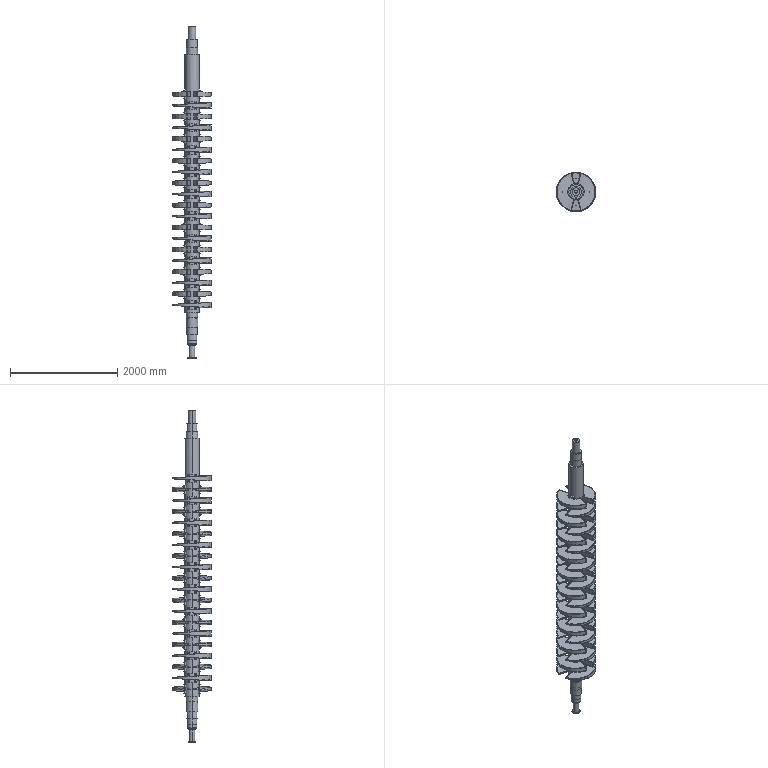Part | SolidWorks | features ReferencePattern 36, LocalLPattern 4, CompositeCurve 2, AEMSimFeature 1, RefAxis 1 | 328 solids | 3332 faces | volume 286429521 mm3 | cylinder 1314 | plane 1274 | spline 720 | cone 20 | torus 4 | commonest cylinder face diameters 18 x320 85 x162 20 x120 50 x82 15 x80 19 x80